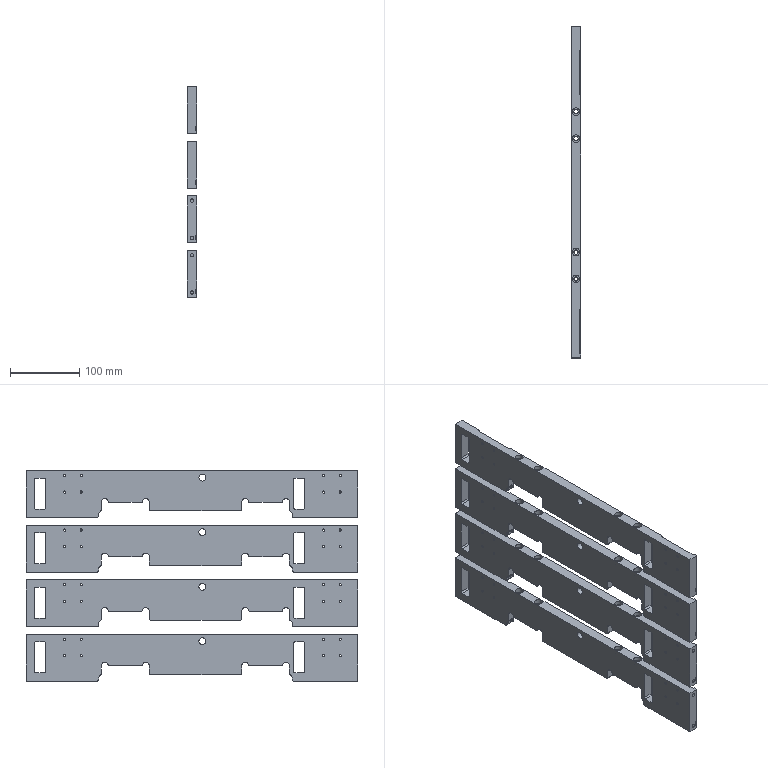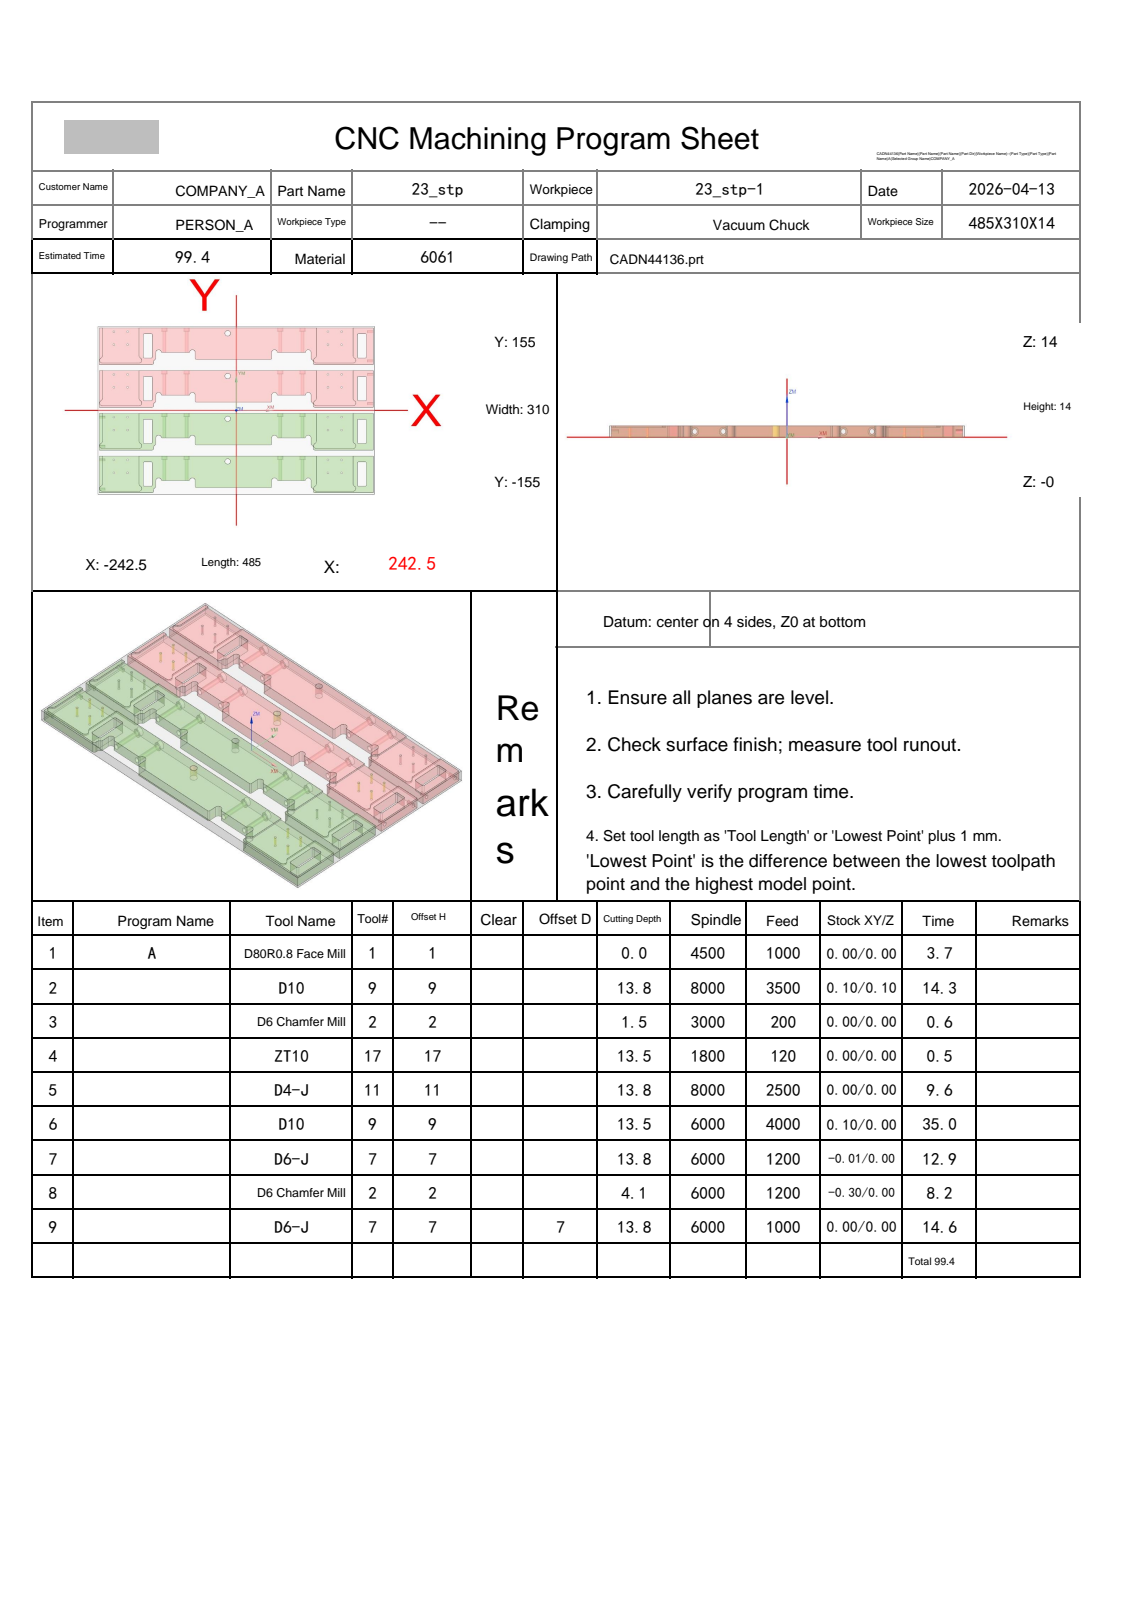NC program | NX | posted by the shop | part box 14 x 480 x 305 mm
Lines 45926 to 46741 of 51894:
N6 T09 M06
(D10  D=10. R=0. H=09 ce=0.10 di=0.00)
G00 G90 G54 X0.0 Y-79.4 M03 S6000
G43 H09 Z34.
M08
Z14.5
G01 X240. Z14.401 F4000.
G02 X245.1 Y-84.5 Z14.397 I0.0 J-5.1
G01 Y-152.5 Z14.369
G02 X240. Y-157.6 Z14.366 I-5.1 J0.0
G01 X138. Z14.323
G02 X129.9 Y-149.5 Z14.318 I0.0 J8.1
G01 Y-147.56 Z14.317
G02 X126. Y-141.222 Z14.314 I3.2 J6.338
G01 Y-130.594 Z14.31
G02 X125.706 Y-131.296 Z14.309 I-6.225 J2.194
X119.775 Y-135. Z14.306 I-5.931 J2.896
G01 X73.225 Z14.287
G02 X67.519 Y-131.717 Z14.284 I0.0 J6.6
X67. Y-130.594 Z14.284 I5.706 J3.317
G01 Y-140.9 Z14.279
G02 X59.9 Y-148. Z14.275 I-7.1 J0.0
G01 X-69.9 Z14.221
G02 X-77. Y-140.9 Z14.216 I0.0 J7.1
G01 Y-130.594 Z14.212
G02 X-77.294 Y-131.296 Z14.212 I-6.225 J2.194
X-83.225 Y-135. Z14.209 I-5.931 J2.896
G01 X-129.775 Z14.189
G02 X-136. Y-130.594 Z14.186 I0.0 J6.6
G01 Y-141.222 Z14.182
G02 X-139.9 Y-147.56 Z14.178 I-7.1 J0.0
G01 Y-149.5
G02 X-148. Y-157.6 Z14.172 I-8.1 J0.0
G01 X-240. Z14.134
G02 X-245.1 Y-152.5 Z14.131 I0.0 J5.1
G01 Y-84.5 Z14.103
G02 X-240. Y-79.4 Z14.099 I5.1 J0.0
G01 X240. Z13.901
G02 X245.1 Y-84.5 Z13.897 I0.0 J-5.1
G01 Y-152.5 Z13.869
G02 X240. Y-157.6 Z13.866 I-5.1 J0.0
G01 X138. Z13.823
G02 X129.9 Y-149.5 Z13.818 I0.0 J8.1
G01 Y-147.56 Z13.817
G02 X126. Y-141.222 Z13.814 I3.2 J6.338
G01 Y-130.594 Z13.81
G02 X125.706 Y-131.296 Z13.809 I-6.225 J2.194
X119.775 Y-135. Z13.806 I-5.931 J2.896
G01 X73.225 Z13.787
G02 X67.519 Y-131.717 Z13.784 I0.0 J6.6
X67. Y-130.594 Z13.784 I5.706 J3.317
G01 Y-140.9 Z13.779
G02 X59.9 Y-148. Z13.775 I-7.1 J0.0
G01 X-69.9 Z13.721
G02 X-77. Y-140.9 Z13.716 I0.0 J7.1
G01 Y-130.594 Z13.712
G02 X-77.294 Y-131.296 Z13.712 I-6.225 J2.194
X-83.225 Y-135. Z13.709 I-5.931 J2.896
G01 X-129.775 Z13.689
G02 X-136. Y-130.594 Z13.686 I0.0 J6.6
G01 Y-141.222 Z13.682
G02 X-139.9 Y-147.56 Z13.678 I-7.1 J0.0
G01 Y-149.5
G02 X-148. Y-157.6 Z13.672 I-8.1 J0.0
G01 X-240. Z13.634
G02 X-245.1 Y-152.5 Z13.631 I0.0 J5.1
G01 Y-84.5 Z13.603
G02 X-240. Y-79.4 Z13.599 I5.1 J0.0
G01 X240. Z13.401
G02 X245.1 Y-84.5 Z13.397 I0.0 J-5.1
G01 Y-152.5 Z13.369
G02 X240. Y-157.6 Z13.366 I-5.1 J0.0
G01 X138. Z13.323
G02 X129.9 Y-149.5 Z13.318 I0.0 J8.1
G01 Y-147.56 Z13.317
G02 X126. Y-141.222 Z13.314 I3.2 J6.338
G01 Y-130.594 Z13.31
G02 X125.706 Y-131.296 Z13.309 I-6.225 J2.194
X119.775 Y-135. Z13.306 I-5.931 J2.896
G01 X73.225 Z13.287
G02 X67.519 Y-131.717 Z13.284 I0.0 J6.6
X67. Y-130.594 Z13.284 I5.706 J3.317
G01 Y-140.9 Z13.279
G02 X59.9 Y-148. Z13.275 I-7.1 J0.0
G01 X-69.9 Z13.221
G02 X-77. Y-140.9 Z13.216 I0.0 J7.1
G01 Y-130.594 Z13.212
G02 X-77.294 Y-131.296 Z13.212 I-6.225 J2.194
X-83.225 Y-135. Z13.209 I-5.931 J2.896
G01 X-129.775 Z13.189
G02 X-136. Y-130.594 Z13.186 I0.0 J6.6
G01 Y-141.222 Z13.182
G02 X-139.9 Y-147.56 Z13.178 I-7.1 J0.0
G01 Y-149.5
G02 X-148. Y-157.6 Z13.172 I-8.1 J0.0
G01 X-240. Z13.134
G02 X-245.1 Y-152.5 Z13.131 I0.0 J5.1
G01 Y-84.5 Z13.103
G02 X-240. Y-79.4 Z13.099 I5.1 J0.0
G01 X240. Z12.901
G02 X245.1 Y-84.5 Z12.897 I0.0 J-5.1
G01 Y-152.5 Z12.869
G02 X240. Y-157.6 Z12.866 I-5.1 J0.0
G01 X138. Z12.823
G02 X129.9 Y-149.5 Z12.818 I0.0 J8.1
G01 Y-147.56 Z12.817
G02 X126. Y-141.222 Z12.814 I3.2 J6.338
G01 Y-130.594 Z12.81
G02 X125.706 Y-131.296 Z12.809 I-6.225 J2.194
X119.775 Y-135. Z12.806 I-5.931 J2.896
G01 X73.225 Z12.787
G02 X67.519 Y-131.717 Z12.784 I0.0 J6.6
X67. Y-130.594 Z12.784 I5.706 J3.317
G01 Y-140.9 Z12.779
G02 X59.9 Y-148. Z12.775 I-7.1 J0.0
G01 X-69.9 Z12.721
G02 X-77. Y-140.9 Z12.716 I0.0 J7.1
G01 Y-130.594 Z12.712
G02 X-77.294 Y-131.296 Z12.712 I-6.225 J2.194
X-83.225 Y-135. Z12.709 I-5.931 J2.896
G01 X-129.775 Z12.689
G02 X-136. Y-130.594 Z12.686 I0.0 J6.6
G01 Y-141.222 Z12.682
G02 X-139.9 Y-147.56 Z12.678 I-7.1 J0.0
G01 Y-149.5
G02 X-148. Y-157.6 Z12.672 I-8.1 J0.0
G01 X-240. Z12.634
G02 X-245.1 Y-152.5 Z12.631 I0.0 J5.1
G01 Y-84.5 Z12.603
G02 X-240. Y-79.4 Z12.599 I5.1 J0.0
G01 X240. Z12.401
G02 X245.1 Y-84.5 Z12.397 I0.0 J-5.1
G01 Y-152.5 Z12.369
G02 X240. Y-157.6 Z12.366 I-5.1 J0.0
G01 X138. Z12.323
G02 X129.9 Y-149.5 Z12.318 I0.0 J8.1
G01 Y-147.56 Z12.317
G02 X126. Y-141.222 Z12.314 I3.2 J6.338
G01 Y-130.594 Z12.31
G02 X125.706 Y-131.296 Z12.309 I-6.225 J2.194
X119.775 Y-135. Z12.306 I-5.931 J2.896
G01 X73.225 Z12.287
G02 X67.519 Y-131.717 Z12.284 I0.0 J6.6
X67. Y-130.594 Z12.284 I5.706 J3.317
G01 Y-140.9 Z12.279
G02 X59.9 Y-148. Z12.275 I-7.1 J0.0
G01 X-69.9 Z12.221
G02 X-77. Y-140.9 Z12.216 I0.0 J7.1
G01 Y-130.594 Z12.212
G02 X-77.294 Y-131.296 Z12.212 I-6.225 J2.194
X-83.225 Y-135. Z12.209 I-5.931 J2.896
G01 X-129.775 Z12.189
G02 X-136. Y-130.594 Z12.186 I0.0 J6.6
G01 Y-141.222 Z12.182
G02 X-139.9 Y-147.56 Z12.178 I-7.1 J0.0
G01 Y-149.5
G02 X-148. Y-157.6 Z12.172 I-8.1 J0.0
G01 X-240. Z12.134
G02 X-245.1 Y-152.5 Z12.131 I0.0 J5.1
G01 Y-84.5 Z12.103
G02 X-240. Y-79.4 Z12.099 I5.1 J0.0
G01 X240. Z11.901
G02 X245.1 Y-84.5 Z11.897 I0.0 J-5.1
G01 Y-152.5 Z11.869
G02 X240. Y-157.6 Z11.866 I-5.1 J0.0
G01 X138. Z11.823
G02 X129.9 Y-149.5 Z11.818 I0.0 J8.1
G01 Y-147.56 Z11.817
G02 X126. Y-141.222 Z11.814 I3.2 J6.338
G01 Y-130.594 Z11.81
G02 X125.706 Y-131.296 Z11.809 I-6.225 J2.194
X119.775 Y-135. Z11.806 I-5.931 J2.896
G01 X73.225 Z11.787
G02 X67.519 Y-131.717 Z11.784 I0.0 J6.6
X67. Y-130.594 Z11.784 I5.706 J3.317
G01 Y-140.9 Z11.779
G02 X59.9 Y-148. Z11.775 I-7.1 J0.0
G01 X-69.9 Z11.721
G02 X-77. Y-140.9 Z11.716 I0.0 J7.1
G01 Y-130.594 Z11.712
G02 X-77.294 Y-131.296 Z11.712 I-6.225 J2.194
X-83.225 Y-135. Z11.709 I-5.931 J2.896
G01 X-129.775 Z11.689
G02 X-136. Y-130.594 Z11.686 I0.0 J6.6
G01 Y-141.222 Z11.682
G02 X-139.9 Y-147.56 Z11.678 I-7.1 J0.0
G01 Y-149.5
G02 X-148. Y-157.6 Z11.672 I-8.1 J0.0
G01 X-240. Z11.634
G02 X-245.1 Y-152.5 Z11.631 I0.0 J5.1
G01 Y-84.5 Z11.603
G02 X-240. Y-79.4 Z11.599 I5.1 J0.0
G01 X240. Z11.401
G02 X245.1 Y-84.5 Z11.397 I0.0 J-5.1
G01 Y-152.5 Z11.369
G02 X240. Y-157.6 Z11.366 I-5.1 J0.0
G01 X138. Z11.323
G02 X129.9 Y-149.5 Z11.318 I0.0 J8.1
G01 Y-147.56 Z11.317
G02 X126. Y-141.222 Z11.314 I3.2 J6.338
G01 Y-130.594 Z11.31
G02 X125.706 Y-131.296 Z11.309 I-6.225 J2.194
X119.775 Y-135. Z11.306 I-5.931 J2.896
G01 X73.225 Z11.287
G02 X67.519 Y-131.717 Z11.284 I0.0 J6.6
X67. Y-130.594 Z11.284 I5.706 J3.317
G01 Y-140.9 Z11.279
G02 X59.9 Y-148. Z11.275 I-7.1 J0.0
G01 X-69.9 Z11.221
G02 X-77. Y-140.9 Z11.216 I0.0 J7.1
G01 Y-130.594 Z11.212
G02 X-77.294 Y-131.296 Z11.212 I-6.225 J2.194
X-83.225 Y-135. Z11.209 I-5.931 J2.896
G01 X-129.775 Z11.189
G02 X-136. Y-130.594 Z11.186 I0.0 J6.6
G01 Y-141.222 Z11.182
G02 X-139.9 Y-147.56 Z11.178 I-7.1 J0.0
G01 Y-149.5
G02 X-148. Y-157.6 Z11.172 I-8.1 J0.0
G01 X-240. Z11.134
G02 X-245.1 Y-152.5 Z11.131 I0.0 J5.1
G01 Y-84.5 Z11.103
G02 X-240. Y-79.4 Z11.099 I5.1 J0.0
G01 X240. Z10.901
G02 X245.1 Y-84.5 Z10.897 I0.0 J-5.1
G01 Y-152.5 Z10.869
G02 X240. Y-157.6 Z10.866 I-5.1 J0.0
G01 X138. Z10.823
G02 X129.9 Y-149.5 Z10.818 I0.0 J8.1
G01 Y-147.56 Z10.817
G02 X126. Y-141.222 Z10.814 I3.2 J6.338
G01 Y-130.594 Z10.81
G02 X125.706 Y-131.296 Z10.809 I-6.225 J2.194
X119.775 Y-135. Z10.806 I-5.931 J2.896
G01 X73.225 Z10.787
G02 X67.519 Y-131.717 Z10.784 I0.0 J6.6
X67. Y-130.594 Z10.784 I5.706 J3.317
G01 Y-140.9 Z10.779
G02 X59.9 Y-148. Z10.775 I-7.1 J0.0
G01 X-69.9 Z10.721
G02 X-77. Y-140.9 Z10.716 I0.0 J7.1
G01 Y-130.594 Z10.712
G02 X-77.294 Y-131.296 Z10.712 I-6.225 J2.194
X-83.225 Y-135. Z10.709 I-5.931 J2.896
G01 X-129.775 Z10.689
G02 X-136. Y-130.594 Z10.686 I0.0 J6.6
G01 Y-141.222 Z10.682
G02 X-139.9 Y-147.56 Z10.678 I-7.1 J0.0
G01 Y-149.5
G02 X-148. Y-157.6 Z10.672 I-8.1 J0.0
G01 X-240. Z10.634
G02 X-245.1 Y-152.5 Z10.631 I0.0 J5.1
G01 Y-84.5 Z10.603
G02 X-240. Y-79.4 Z10.599 I5.1 J0.0
G01 X240. Z10.401
G02 X245.1 Y-84.5 Z10.397 I0.0 J-5.1
G01 Y-152.5 Z10.369
G02 X240. Y-157.6 Z10.366 I-5.1 J0.0
G01 X138. Z10.323
G02 X129.9 Y-149.5 Z10.318 I0.0 J8.1
G01 Y-147.56 Z10.317
G02 X126. Y-141.222 Z10.314 I3.2 J6.338
G01 Y-130.594 Z10.31
G02 X125.706 Y-131.296 Z10.309 I-6.225 J2.194
X119.775 Y-135. Z10.306 I-5.931 J2.896
G01 X73.225 Z10.287
G02 X67.519 Y-131.717 Z10.284 I0.0 J6.6
X67. Y-130.594 Z10.284 I5.706 J3.317
G01 Y-140.9 Z10.279
G02 X59.9 Y-148. Z10.275 I-7.1 J0.0
G01 X-69.9 Z10.221
G02 X-77. Y-140.9 Z10.216 I0.0 J7.1
G01 Y-130.594 Z10.212
G02 X-77.294 Y-131.296 Z10.212 I-6.225 J2.194
X-83.225 Y-135. Z10.209 I-5.931 J2.896
G01 X-129.775 Z10.189
G02 X-136. Y-130.594 Z10.186 I0.0 J6.6
G01 Y-141.222 Z10.182
G02 X-139.9 Y-147.56 Z10.178 I-7.1 J0.0
G01 Y-149.5
G02 X-148. Y-157.6 Z10.172 I-8.1 J0.0
G01 X-240. Z10.134
G02 X-245.1 Y-152.5 Z10.131 I0.0 J5.1
G01 Y-84.5 Z10.103
G02 X-240. Y-79.4 Z10.099 I5.1 J0.0
G01 X240. Z9.901
G02 X245.1 Y-84.5 Z9.897 I0.0 J-5.1
G01 Y-152.5 Z9.869
G02 X240. Y-157.6 Z9.866 I-5.1 J0.0
G01 X138. Z9.823
G02 X129.9 Y-149.5 Z9.818 I0.0 J8.1
G01 Y-147.56 Z9.817
G02 X126. Y-141.222 Z9.814 I3.2 J6.338
G01 Y-130.594 Z9.81
G02 X125.706 Y-131.296 Z9.809 I-6.225 J2.194
X119.775 Y-135. Z9.806 I-5.931 J2.896
G01 X73.225 Z9.787
G02 X67.519 Y-131.717 Z9.784 I0.0 J6.6
X67. Y-130.594 Z9.784 I5.706 J3.317
G01 Y-140.9 Z9.779
G02 X59.9 Y-148. Z9.775 I-7.1 J0.0
G01 X-69.9 Z9.721
G02 X-77. Y-140.9 Z9.716 I0.0 J7.1
G01 Y-130.594 Z9.712
G02 X-77.294 Y-131.296 Z9.712 I-6.225 J2.194
X-83.225 Y-135. Z9.709 I-5.931 J2.896
G01 X-129.775 Z9.689
G02 X-136. Y-130.594 Z9.686 I0.0 J6.6
G01 Y-141.222 Z9.682
G02 X-139.9 Y-147.56 Z9.678 I-7.1 J0.0
G01 Y-149.5
G02 X-148. Y-157.6 Z9.672 I-8.1 J0.0
G01 X-240. Z9.634
G02 X-245.1 Y-152.5 Z9.631 I0.0 J5.1
G01 Y-84.5 Z9.603
G02 X-240. Y-79.4 Z9.599 I5.1 J0.0
G01 X240. Z9.401
G02 X245.1 Y-84.5 Z9.397 I0.0 J-5.1
G01 Y-152.5 Z9.369
G02 X240. Y-157.6 Z9.366 I-5.1 J0.0
G01 X138. Z9.323
G02 X129.9 Y-149.5 Z9.318 I0.0 J8.1
G01 Y-147.56 Z9.317
G02 X126. Y-141.222 Z9.314 I3.2 J6.338
G01 Y-130.594 Z9.31
G02 X125.706 Y-131.296 Z9.309 I-6.225 J2.194
X119.775 Y-135. Z9.306 I-5.931 J2.896
G01 X73.225 Z9.287
G02 X67.519 Y-131.717 Z9.284 I0.0 J6.6
X67. Y-130.594 Z9.284 I5.706 J3.317
G01 Y-140.9 Z9.279
G02 X59.9 Y-148. Z9.275 I-7.1 J0.0
G01 X-69.9 Z9.221
G02 X-77. Y-140.9 Z9.216 I0.0 J7.1
G01 Y-130.594 Z9.212
G02 X-77.294 Y-131.296 Z9.212 I-6.225 J2.194
X-83.225 Y-135. Z9.209 I-5.931 J2.896
G01 X-129.775 Z9.189
G02 X-136. Y-130.594 Z9.186 I0.0 J6.6
G01 Y-141.222 Z9.182
G02 X-139.9 Y-147.56 Z9.178 I-7.1 J0.0
G01 Y-149.5
G02 X-148. Y-157.6 Z9.172 I-8.1 J0.0
G01 X-240. Z9.134
G02 X-245.1 Y-152.5 Z9.131 I0.0 J5.1
G01 Y-84.5 Z9.103
G02 X-240. Y-79.4 Z9.099 I5.1 J0.0
G01 X240. Z8.901
G02 X245.1 Y-84.5 Z8.897 I0.0 J-5.1
G01 Y-152.5 Z8.869
G02 X240. Y-157.6 Z8.866 I-5.1 J0.0
G01 X138. Z8.823
G02 X129.9 Y-149.5 Z8.818 I0.0 J8.1
G01 Y-147.56 Z8.817
G02 X126. Y-141.222 Z8.814 I3.2 J6.338
G01 Y-130.594 Z8.81
G02 X125.706 Y-131.296 Z8.809 I-6.225 J2.194
X119.775 Y-135. Z8.806 I-5.931 J2.896
G01 X73.225 Z8.787
G02 X67.519 Y-131.717 Z8.784 I0.0 J6.6
X67. Y-130.594 Z8.784 I5.706 J3.317
G01 Y-140.9 Z8.779
G02 X59.9 Y-148. Z8.775 I-7.1 J0.0
G01 X-69.9 Z8.721
G02 X-77. Y-140.9 Z8.716 I0.0 J7.1
G01 Y-130.594 Z8.712
G02 X-77.294 Y-131.296 Z8.712 I-6.225 J2.194
X-83.225 Y-135. Z8.709 I-5.931 J2.896
G01 X-129.775 Z8.689
G02 X-136. Y-130.594 Z8.686 I0.0 J6.6
G01 Y-141.222 Z8.682
G02 X-139.9 Y-147.56 Z8.678 I-7.1 J0.0
G01 Y-149.5
G02 X-148. Y-157.6 Z8.672 I-8.1 J0.0
G01 X-240. Z8.634
G02 X-245.1 Y-152.5 Z8.631 I0.0 J5.1
G01 Y-84.5 Z8.603
G02 X-240. Y-79.4 Z8.599 I5.1 J0.0
G01 X240. Z8.401
G02 X245.1 Y-84.5 Z8.397 I0.0 J-5.1
G01 Y-152.5 Z8.369
G02 X240. Y-157.6 Z8.366 I-5.1 J0.0
G01 X138. Z8.323
G02 X129.9 Y-149.5 Z8.318 I0.0 J8.1
G01 Y-147.56 Z8.317
G02 X126. Y-141.222 Z8.314 I3.2 J6.338
G01 Y-130.594 Z8.31
G02 X125.706 Y-131.296 Z8.309 I-6.225 J2.194
X119.775 Y-135. Z8.306 I-5.931 J2.896
G01 X73.225 Z8.287
G02 X67.519 Y-131.717 Z8.284 I0.0 J6.6
X67. Y-130.594 Z8.284 I5.706 J3.317
G01 Y-140.9 Z8.279
G02 X59.9 Y-148. Z8.275 I-7.1 J0.0
G01 X-69.9 Z8.221
G02 X-77. Y-140.9 Z8.216 I0.0 J7.1
G01 Y-130.594 Z8.212
G02 X-77.294 Y-131.296 Z8.212 I-6.225 J2.194
X-83.225 Y-135. Z8.209 I-5.931 J2.896
G01 X-129.775 Z8.189
G02 X-136. Y-130.594 Z8.186 I0.0 J6.6
G01 Y-141.222 Z8.182
G02 X-139.9 Y-147.56 Z8.178 I-7.1 J0.0
G01 Y-149.5
G02 X-148. Y-157.6 Z8.172 I-8.1 J0.0
G01 X-240. Z8.134
G02 X-245.1 Y-152.5 Z8.131 I0.0 J5.1
G01 Y-84.5 Z8.103
G02 X-240. Y-79.4 Z8.099 I5.1 J0.0
G01 X240. Z7.901
G02 X245.1 Y-84.5 Z7.897 I0.0 J-5.1
G01 Y-152.5 Z7.869
G02 X240. Y-157.6 Z7.866 I-5.1 J0.0
G01 X138. Z7.823
G02 X129.9 Y-149.5 Z7.818 I0.0 J8.1
G01 Y-147.56 Z7.817
G02 X126. Y-141.222 Z7.814 I3.2 J6.338
G01 Y-130.594 Z7.81
G02 X125.706 Y-131.296 Z7.809 I-6.225 J2.194
X119.775 Y-135. Z7.806 I-5.931 J2.896
G01 X73.225 Z7.787
G02 X67.519 Y-131.717 Z7.784 I0.0 J6.6
X67. Y-130.594 Z7.784 I5.706 J3.317
G01 Y-140.9 Z7.779
G02 X59.9 Y-148. Z7.775 I-7.1 J0.0
G01 X-69.9 Z7.721
G02 X-77. Y-140.9 Z7.716 I0.0 J7.1
G01 Y-130.594 Z7.712
G02 X-77.294 Y-131.296 Z7.712 I-6.225 J2.194
X-83.225 Y-135. Z7.709 I-5.931 J2.896
G01 X-129.775 Z7.689
G02 X-136. Y-130.594 Z7.686 I0.0 J6.6
G01 Y-141.222 Z7.682
G02 X-139.9 Y-147.56 Z7.678 I-7.1 J0.0
G01 Y-149.5
G02 X-148. Y-157.6 Z7.672 I-8.1 J0.0
G01 X-240. Z7.634
G02 X-245.1 Y-152.5 Z7.631 I0.0 J5.1
G01 Y-84.5 Z7.603
G02 X-240. Y-79.4 Z7.599 I5.1 J0.0
G01 X240. Z7.401
G02 X245.1 Y-84.5 Z7.397 I0.0 J-5.1
G01 Y-152.5 Z7.369
G02 X240. Y-157.6 Z7.366 I-5.1 J0.0
G01 X138. Z7.323
G02 X129.9 Y-149.5 Z7.318 I0.0 J8.1
G01 Y-147.56 Z7.317
G02 X126. Y-141.222 Z7.314 I3.2 J6.338
G01 Y-130.594 Z7.31
G02 X125.706 Y-131.296 Z7.309 I-6.225 J2.194
X119.775 Y-135. Z7.306 I-5.931 J2.896
G01 X73.225 Z7.287
G02 X67.519 Y-131.717 Z7.284 I0.0 J6.6
X67. Y-130.594 Z7.284 I5.706 J3.317
G01 Y-140.9 Z7.279
G02 X59.9 Y-148. Z7.275 I-7.1 J0.0
G01 X-69.9 Z7.221
G02 X-77. Y-140.9 Z7.216 I0.0 J7.1
G01 Y-130.594 Z7.212
G02 X-77.294 Y-131.296 Z7.212 I-6.225 J2.194
X-83.225 Y-135. Z7.209 I-5.931 J2.896
G01 X-129.775 Z7.189
G02 X-136. Y-130.594 Z7.186 I0.0 J6.6
G01 Y-141.222 Z7.182
G02 X-139.9 Y-147.56 Z7.178 I-7.1 J0.0
G01 Y-149.5
G02 X-148. Y-157.6 Z7.172 I-8.1 J0.0
G01 X-240. Z7.134
G02 X-245.1 Y-152.5 Z7.131 I0.0 J5.1
G01 Y-84.5 Z7.103
G02 X-240. Y-79.4 Z7.099 I5.1 J0.0
G01 X240. Z6.901
G02 X245.1 Y-84.5 Z6.897 I0.0 J-5.1
G01 Y-152.5 Z6.869
G02 X240. Y-157.6 Z6.866 I-5.1 J0.0
G01 X138. Z6.823
G02 X129.9 Y-149.5 Z6.818 I0.0 J8.1
G01 Y-147.56 Z6.817
G02 X126. Y-141.222 Z6.814 I3.2 J6.338
G01 Y-130.594 Z6.81
G02 X125.706 Y-131.296 Z6.809 I-6.225 J2.194
X119.775 Y-135. Z6.806 I-5.931 J2.896
G01 X73.225 Z6.787
G02 X67.519 Y-131.717 Z6.784 I0.0 J6.6
X67. Y-130.594 Z6.784 I5.706 J3.317
G01 Y-140.9 Z6.779
G02 X59.9 Y-148. Z6.775 I-7.1 J0.0
G01 X-69.9 Z6.721
G02 X-77. Y-140.9 Z6.716 I0.0 J7.1
G01 Y-130.594 Z6.712
G02 X-77.294 Y-131.296 Z6.712 I-6.225 J2.194
X-83.225 Y-135. Z6.709 I-5.931 J2.896
G01 X-129.775 Z6.689
G02 X-136. Y-130.594 Z6.686 I0.0 J6.6
G01 Y-141.222 Z6.682
G02 X-139.9 Y-147.56 Z6.678 I-7.1 J0.0
G01 Y-149.5
G02 X-148. Y-157.6 Z6.672 I-8.1 J0.0
G01 X-240. Z6.634
G02 X-245.1 Y-152.5 Z6.631 I0.0 J5.1
G01 Y-84.5 Z6.603
G02 X-240. Y-79.4 Z6.599 I5.1 J0.0
G01 X240. Z6.401
G02 X245.1 Y-84.5 Z6.397 I0.0 J-5.1
G01 Y-152.5 Z6.369
G02 X240. Y-157.6 Z6.366 I-5.1 J0.0
G01 X138. Z6.323
G02 X129.9 Y-149.5 Z6.318 I0.0 J8.1
G01 Y-147.56 Z6.317
G02 X126. Y-141.222 Z6.314 I3.2 J6.338
G01 Y-130.594 Z6.31
G02 X125.706 Y-131.296 Z6.309 I-6.225 J2.194
X119.775 Y-135. Z6.306 I-5.931 J2.896
G01 X73.225 Z6.287
G02 X67.519 Y-131.717 Z6.284 I0.0 J6.6
X67. Y-130.594 Z6.284 I5.706 J3.317
G01 Y-140.9 Z6.279
G02 X59.9 Y-148. Z6.275 I-7.1 J0.0
G01 X-69.9 Z6.221
G02 X-77. Y-140.9 Z6.216 I0.0 J7.1
G01 Y-130.594 Z6.212
G02 X-77.294 Y-131.296 Z6.212 I-6.225 J2.194
X-83.225 Y-135. Z6.209 I-5.931 J2.896
G01 X-129.775 Z6.189
G02 X-136. Y-130.594 Z6.186 I0.0 J6.6
G01 Y-141.222 Z6.182
G02 X-139.9 Y-147.56 Z6.178 I-7.1 J0.0
G01 Y-149.5
G02 X-148. Y-157.6 Z6.172 I-8.1 J0.0
G01 X-240. Z6.134
G02 X-245.1 Y-152.5 Z6.131 I0.0 J5.1
G01 Y-84.5 Z6.103
G02 X-240. Y-79.4 Z6.099 I5.1 J0.0
G01 X240. Z5.901
G02 X245.1 Y-84.5 Z5.897 I0.0 J-5.1
G01 Y-152.5 Z5.869
G02 X240. Y-157.6 Z5.866 I-5.1 J0.0
G01 X138. Z5.823
G02 X129.9 Y-149.5 Z5.818 I0.0 J8.1
G01 Y-147.56 Z5.817
G02 X126. Y-141.222 Z5.814 I3.2 J6.338
G01 Y-130.594 Z5.81
G02 X125.706 Y-131.296 Z5.809 I-6.225 J2.194
X119.775 Y-135. Z5.806 I-5.931 J2.896
G01 X73.225 Z5.787
G02 X67.519 Y-131.717 Z5.784 I0.0 J6.6
X67. Y-130.594 Z5.784 I5.706 J3.317
G01 Y-140.9 Z5.779
G02 X59.9 Y-148. Z5.775 I-7.1 J0.0
G01 X-69.9 Z5.721
G02 X-77. Y-140.9 Z5.716 I0.0 J7.1
G01 Y-130.594 Z5.712
G02 X-77.294 Y-131.296 Z5.712 I-6.225 J2.194
X-83.225 Y-135. Z5.709 I-5.931 J2.896
G01 X-129.775 Z5.689
G02 X-136. Y-130.594 Z5.686 I0.0 J6.6
G01 Y-141.222 Z5.682
G02 X-139.9 Y-147.56 Z5.678 I-7.1 J0.0
G01 Y-149.5
G02 X-148. Y-157.6 Z5.672 I-8.1 J0.0
G01 X-240. Z5.634
G02 X-245.1 Y-152.5 Z5.631 I0.0 J5.1
G01 Y-84.5 Z5.603
G02 X-240. Y-79.4 Z5.599 I5.1 J0.0
G01 X240. Z5.401
G02 X245.1 Y-84.5 Z5.397 I0.0 J-5.1
G01 Y-152.5 Z5.369
G02 X240. Y-157.6 Z5.366 I-5.1 J0.0
G01 X138. Z5.323
G02 X129.9 Y-149.5 Z5.318 I0.0 J8.1
G01 Y-147.56 Z5.317
G02 X126. Y-141.222 Z5.314 I3.2 J6.338
G01 Y-130.594 Z5.31
G02 X125.706 Y-131.296 Z5.309 I-6.225 J2.194
X119.775 Y-135. Z5.306 I-5.931 J2.896
G01 X73.225 Z5.287
G02 X67.519 Y-131.717 Z5.284 I0.0 J6.6
X67. Y-130.594 Z5.284 I5.706 J3.317
G01 Y-140.9 Z5.279
G02 X59.9 Y-148. Z5.275 I-7.1 J0.0
G01 X-69.9 Z5.221
G02 X-77. Y-140.9 Z5.216 I0.0 J7.1
G01 Y-130.594 Z5.212
G02 X-77.294 Y-131.296 Z5.212 I-6.225 J2.194
X-83.225 Y-135. Z5.209 I-5.931 J2.896
G01 X-129.775 Z5.189
G02 X-136. Y-130.594 Z5.186 I0.0 J6.6
G01 Y-141.222 Z5.182
G02 X-139.9 Y-147.56 Z5.178 I-7.1 J0.0
G01 Y-149.5
G02 X-148. Y-157.6 Z5.172 I-8.1 J0.0
G01 X-240. Z5.134
G02 X-245.1 Y-152.5 Z5.131 I0.0 J5.1
G01 Y-84.5 Z5.103
G02 X-240. Y-79.4 Z5.099 I5.1 J0.0
G01 X240. Z4.901
G02 X245.1 Y-84.5 Z4.897 I0.0 J-5.1
G01 Y-152.5 Z4.869
G02 X240. Y-157.6 Z4.866 I-5.1 J0.0
G01 X138. Z4.823
G02 X129.9 Y-149.5 Z4.818 I0.0 J8.1
G01 Y-147.56 Z4.817
G02 X126. Y-141.222 Z4.814 I3.2 J6.338
G01 Y-130.594 Z4.81
G02 X125.706 Y-131.296 Z4.809 I-6.225 J2.194
X119.775 Y-135. Z4.806 I-5.931 J2.896
G01 X73.225 Z4.787
G02 X67.519 Y-131.717 Z4.784 I0.0 J6.6
X67. Y-130.594 Z4.784 I5.706 J3.317
G01 Y-140.9 Z4.779
G02 X59.9 Y-148. Z4.775 I-7.1 J0.0
G01 X-69.9 Z4.721
G02 X-77. Y-140.9 Z4.716 I0.0 J7.1
G01 Y-130.594 Z4.712
G02 X-77.294 Y-131.296 Z4.712 I-6.225 J2.194
X-83.225 Y-135. Z4.709 I-5.931 J2.896
G01 X-129.775 Z4.689
G02 X-136. Y-130.594 Z4.686 I0.0 J6.6
G01 Y-141.222 Z4.682
G02 X-139.9 Y-147.56 Z4.678 I-7.1 J0.0
G01 Y-149.5
G02 X-148. Y-157.6 Z4.672 I-8.1 J0.0
G01 X-240. Z4.634
G02 X-245.1 Y-152.5 Z4.631 I0.0 J5.1
G01 Y-84.5 Z4.603
G02 X-240. Y-79.4 Z4.599 I5.1 J0.0
G01 X240. Z4.401
G02 X245.1 Y-84.5 Z4.397 I0.0 J-5.1
G01 Y-152.5 Z4.369
G02 X240. Y-157.6 Z4.366 I-5.1 J0.0
G01 X138. Z4.323
G02 X129.9 Y-149.5 Z4.318 I0.0 J8.1
G01 Y-147.56 Z4.317
G02 X126. Y-141.222 Z4.314 I3.2 J6.338
G01 Y-130.594 Z4.31
G02 X125.706 Y-131.296 Z4.309 I-6.225 J2.194
X119.775 Y-135. Z4.306 I-5.931 J2.896
G01 X73.225 Z4.287
G02 X67.519 Y-131.717 Z4.284 I0.0 J6.6
X67. Y-130.594 Z4.284 I5.706 J3.317
G01 Y-140.9 Z4.279
G02 X59.9 Y-148. Z4.275 I-7.1 J0.0
G01 X-69.9 Z4.221
G02 X-77. Y-140.9 Z4.216 I0.0 J7.1
G01 Y-130.594 Z4.212
G02 X-77.294 Y-131.296 Z4.212 I-6.225 J2.194
X-83.225 Y-135. Z4.209 I-5.931 J2.896
G01 X-129.775 Z4.189
G02 X-136. Y-130.594 Z4.186 I0.0 J6.6
G01 Y-141.222 Z4.182
G02 X-139.9 Y-147.56 Z4.178 I-7.1 J0.0
G01 Y-149.5
G02 X-148. Y-157.6 Z4.172 I-8.1 J0.0
G01 X-240. Z4.134
G02 X-245.1 Y-152.5 Z4.131 I0.0 J5.1
G01 Y-84.5 Z4.103
G02 X-240. Y-79.4 Z4.099 I5.1 J0.0
G01 X240. Z3.901
G02 X245.1 Y-84.5 Z3.897 I0.0 J-5.1
G01 Y-152.5 Z3.869
G02 X240. Y-157.6 Z3.866 I-5.1 J0.0
G01 X138. Z3.823
G02 X129.9 Y-149.5 Z3.818 I0.0 J8.1
G01 Y-147.56 Z3.817
G02 X126. Y-141.222 Z3.814 I3.2 J6.338
G01 Y-130.594 Z3.81
G02 X125.706 Y-131.296 Z3.809 I-6.225 J2.194
X119.775 Y-135. Z3.806 I-5.931 J2.896
G01 X73.225 Z3.787
G02 X67.519 Y-131.717 Z3.784 I0.0 J6.6
X67. Y-130.594 Z3.784 I5.706 J3.317
G01 Y-140.9 Z3.779
G02 X59.9 Y-148. Z3.775 I-7.1 J0.0
G01 X-69.9 Z3.721
G02 X-77. Y-140.9 Z3.716 I0.0 J7.1
G01 Y-130.594 Z3.712
G02 X-77.294 Y-131.296 Z3.712 I-6.225 J2.194
X-83.225 Y-135. Z3.709 I-5.931 J2.896
G01 X-129.775 Z3.689
G02 X-136. Y-130.594 Z3.686 I0.0 J6.6
G01 Y-141.222 Z3.682
G02 X-139.9 Y-147.56 Z3.678 I-7.1 J0.0
G01 Y-149.5
G02 X-148. Y-157.6 Z3.672 I-8.1 J0.0
G01 X-240. Z3.634
G02 X-245.1 Y-152.5 Z3.631 I0.0 J5.1
G01 Y-84.5 Z3.603
G02 X-240. Y-79.4 Z3.599 I5.1 J0.0
G01 X240. Z3.401
G02 X245.1 Y-84.5 Z3.397 I0.0 J-5.1
G01 Y-152.5 Z3.369
G02 X240. Y-157.6 Z3.366 I-5.1 J0.0
G01 X138. Z3.323
G02 X129.9 Y-149.5 Z3.318 I0.0 J8.1
G01 Y-147.56 Z3.317
G02 X126. Y-141.222 Z3.314 I3.2 J6.338
G01 Y-130.594 Z3.31
G02 X125.706 Y-131.296 Z3.309 I-6.225 J2.194
X119.775 Y-135. Z3.306 I-5.931 J2.896
G01 X73.225 Z3.287
G02 X67.519 Y-131.717 Z3.284 I0.0 J6.6
X67. Y-130.594 Z3.284 I5.706 J3.317
G01 Y-140.9 Z3.279
G02 X59.9 Y-148. Z3.275 I-7.1 J0.0
G01 X-69.9 Z3.221
G02 X-77. Y-140.9 Z3.216 I0.0 J7.1
G01 Y-130.594 Z3.212
G02 X-77.294 Y-131.296 Z3.212 I-6.225 J2.194
X-83.225 Y-135. Z3.209 I-5.931 J2.896
G01 X-129.775 Z3.189
G02 X-136. Y-130.594 Z3.186 I0.0 J6.6
G01 Y-141.222 Z3.182
G02 X-139.9 Y-147.56 Z3.178 I-7.1 J0.0
G01 Y-149.5
G02 X-148. Y-157.6 Z3.172 I-8.1 J0.0
G01 X-240. Z3.134
G02 X-245.1 Y-152.5 Z3.131 I0.0 J5.1
G01 Y-84.5 Z3.103
G02 X-240. Y-79.4 Z3.099 I5.1 J0.0
G01 X240. Z2.901
G02 X245.1 Y-84.5 Z2.897 I0.0 J-5.1
G01 Y-152.5 Z2.869
G02 X240. Y-157.6 Z2.866 I-5.1 J0.0
G01 X138. Z2.823
G02 X129.9 Y-149.5 Z2.818 I0.0 J8.1
G01 Y-147.56 Z2.817
G02 X126. Y-141.222 Z2.814 I3.2 J6.338
G01 Y-130.594 Z2.81
G02 X125.706 Y-131.296 Z2.809 I-6.225 J2.194
X119.775 Y-135. Z2.806 I-5.931 J2.896
G01 X73.225 Z2.787
G02 X67.519 Y-131.717 Z2.784 I0.0 J6.6
X67. Y-130.594 Z2.784 I5.706 J3.317
G01 Y-140.9 Z2.779
G02 X59.9 Y-148. Z2.775 I-7.1 J0.0
G01 X-69.9 Z2.721
G02 X-77. Y-140.9 Z2.716 I0.0 J7.1
G01 Y-130.594 Z2.712
G02 X-77.294 Y-131.296 Z2.712 I-6.225 J2.194
X-83.225 Y-135. Z2.709 I-5.931 J2.896
G01 X-129.775 Z2.689
G02 X-136. Y-130.594 Z2.686 I0.0 J6.6
G01 Y-141.222 Z2.682
G02 X-139.9 Y-147.56 Z2.678 I-7.1 J0.0
G01 Y-149.5
G02 X-148. Y-157.6 Z2.672 I-8.1 J0.0
G01 X-240. Z2.634
G02 X-245.1 Y-152.5 Z2.631 I0.0 J5.1
G01 Y-84.5 Z2.603
G02 X-240. Y-79.4 Z2.599 I5.1 J0.0
G01 X240. Z2.401
G02 X245.1 Y-84.5 Z2.397 I0.0 J-5.1
G01 Y-152.5 Z2.369
G02 X240. Y-157.6 Z2.366 I-5.1 J0.0
G01 X138. Z2.323
G02 X129.9 Y-149.5 Z2.318 I0.0 J8.1
G01 Y-147.56 Z2.317
G02 X126. Y-141.222 Z2.314 I3.2 J6.338
G01 Y-130.594 Z2.31
G02 X125.706 Y-131.296 Z2.309 I-6.225 J2.194
X119.775 Y-135. Z2.306 I-5.931 J2.896
G01 X73.225 Z2.287
G02 X67.519 Y-131.717 Z2.284 I0.0 J6.6
X67. Y-130.594 Z2.284 I5.706 J3.317
G01 Y-140.9 Z2.279
G02 X59.9 Y-148. Z2.275 I-7.1 J0.0
G01 X-69.9 Z2.221
G02 X-77. Y-140.9 Z2.216 I0.0 J7.1
G01 Y-130.594 Z2.212
G02 X-77.294 Y-131.296 Z2.212 I-6.225 J2.194
X-83.225 Y-135. Z2.209 I-5.931 J2.896
G01 X-129.775 Z2.189
G02 X-136. Y-130.594 Z2.186 I0.0 J6.6
G01 Y-141.222 Z2.182
G02 X-139.9 Y-147.56 Z2.178 I-7.1 J0.0
G01 Y-149.5
G02 X-148. Y-157.6 Z2.172 I-8.1 J0.0
G01 X-240. Z2.134
G02 X-245.1 Y-152.5 Z2.131 I0.0 J5.1
G01 Y-84.5 Z2.103
G02 X-240. Y-79.4 Z2.099 I5.1 J0.0
G01 X240. Z1.901
G02 X245.1 Y-84.5 Z1.897 I0.0 J-5.1
G01 Y-152.5 Z1.869
G02 X240. Y-157.6 Z1.866 I-5.1 J0.0
G01 X138. Z1.823
G02 X129.9 Y-149.5 Z1.818 I0.0 J8.1
G01 Y-147.56 Z1.817
G02 X126. Y-141.222 Z1.814 I3.2 J6.338
G01 Y-130.594 Z1.81
G02 X125.706 Y-131.296 Z1.809 I-6.225 J2.194
X119.775 Y-135. Z1.806 I-5.931 J2.896
G01 X73.225 Z1.787
G02 X67.519 Y-131.717 Z1.784 I0.0 J6.6
X67. Y-130.594 Z1.784 I5.706 J3.317
G01 Y-140.9 Z1.779
G02 X59.9 Y-148. Z1.775 I-7.1 J0.0
G01 X-69.9 Z1.721
G02 X-77. Y-140.9 Z1.716 I0.0 J7.1
G01 Y-130.594 Z1.712
G02 X-77.294 Y-131.296 Z1.712 I-6.225 J2.194
X-83.225 Y-135. Z1.709 I-5.931 J2.896
G01 X-129.775 Z1.689
G02 X-136. Y-130.594 Z1.686 I0.0 J6.6
G01 Y-141.222 Z1.682
G02 X-139.9 Y-147.56 Z1.678 I-7.1 J0.0
G01 Y-149.5
G02 X-148. Y-157.6 Z1.672 I-8.1 J0.0
G01 X-240. Z1.634
G02 X-245.1 Y-152.5 Z1.631 I0.0 J5.1
G01 Y-84.5 Z1.603
G02 X-240. Y-79.4 Z1.599 I5.1 J0.0
G01 X240. Z1.401
G02 X245.1 Y-84.5 Z1.397 I0.0 J-5.1
G01 Y-152.5 Z1.369
G02 X240. Y-157.6 Z1.366 I-5.1 J0.0